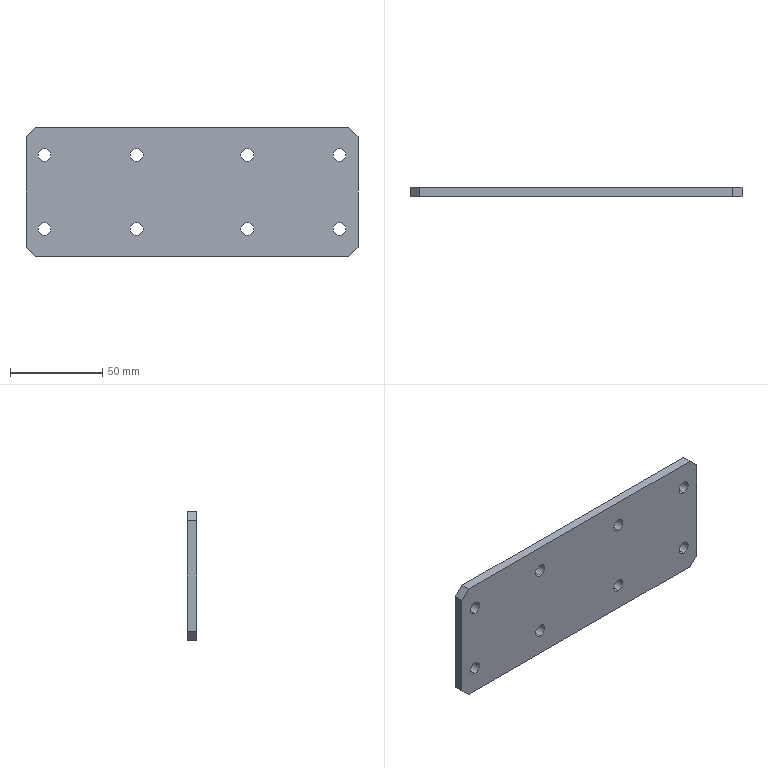Part | NX | features BREP 1 | 1 solid | 26 faces | box 180 x 5 x 70 mm | volume 61211 mm3 | cylinder 16 | plane 10 | commonest cylinder face diameters 7 x16
STEP:
#1=CARTESIAN_POINT('',(85.,5.,35.));
#2=VERTEX_POINT('',#1);
#3=CARTESIAN_POINT('',(90.,5.,30.));
#4=VERTEX_POINT('',#3);
#5=CARTESIAN_POINT('',(60.,5.,60.));
#6=DIRECTION('',(0.7071,0.,-0.7071));
#7=VECTOR('',#6,1000.);
#8=LINE('',#5,#7);
#9=EDGE_CURVE('',#2,#4,#8,.T.);
#10=ORIENTED_EDGE('',*,*,#9,.F.);
#11=CARTESIAN_POINT('',(85.,0.,35.));
#12=VERTEX_POINT('',#11);
#13=CARTESIAN_POINT('',(85.,5.,35.));
#14=DIRECTION('',(0.,1.,0.));
#15=VECTOR('',#14,1000.);
#16=LINE('',#13,#15);
#17=EDGE_CURVE('',#12,#2,#16,.T.);
#18=ORIENTED_EDGE('',*,*,#17,.F.);
#19=CARTESIAN_POINT('',(90.,0.,30.));
#20=VERTEX_POINT('',#19);
#21=CARTESIAN_POINT('',(90.,0.,30.));
#22=DIRECTION('',(-0.7071,0.,0.7071));
#23=VECTOR('',#22,1000.);
#24=LINE('',#21,#23);
#25=EDGE_CURVE('',#20,#12,#24,.T.);
#26=ORIENTED_EDGE('',*,*,#25,.F.);
#27=CARTESIAN_POINT('',(90.,5.,30.));
#28=DIRECTION('',(0.,-1.,0.));
#29=VECTOR('',#28,1000.);
#30=LINE('',#27,#29);
#31=EDGE_CURVE('',#4,#20,#30,.T.);
#32=ORIENTED_EDGE('',*,*,#31,.F.);
#33=EDGE_LOOP('',(#10,#18,#26,#32));
#34=FACE_BOUND('',#33,.T.);
#35=CARTESIAN_POINT('',(90.,5.,30.));
#36=DIRECTION('',(-0.7071,0.,-0.7071));
#37=DIRECTION('',(0.,-1.,0.));
#38=AXIS2_PLACEMENT_3D('',#35,#36,#37);
#39=PLANE('',#38);
#40=ADVANCED_FACE('',(#34),#39,.F.);
#41=CARTESIAN_POINT('',(90.,5.,-30.));
#42=VERTEX_POINT('',#41);
#43=CARTESIAN_POINT('',(85.,5.,-35.));
#44=VERTEX_POINT('',#43);
#45=CARTESIAN_POINT('',(60.,5.,-60.));
#46=DIRECTION('',(-0.7071,0.,-0.7071));
#47=VECTOR('',#46,1000.);
#48=LINE('',#45,#47);
#49=EDGE_CURVE('',#42,#44,#48,.T.);
#50=ORIENTED_EDGE('',*,*,#49,.F.);
#51=CARTESIAN_POINT('',(90.,0.,-30.));
#52=VERTEX_POINT('',#51);
#53=CARTESIAN_POINT('',(90.,5.,-30.));
#54=DIRECTION('',(0.,1.,0.));
#55=VECTOR('',#54,1000.);
#56=LINE('',#53,#55);
#57=EDGE_CURVE('',#52,#42,#56,.T.);
#58=ORIENTED_EDGE('',*,*,#57,.F.);
#59=CARTESIAN_POINT('',(85.,0.,-35.));
#60=VERTEX_POINT('',#59);
#61=CARTESIAN_POINT('',(85.,0.,-35.));
#62=DIRECTION('',(0.7071,0.,0.7071));
#63=VECTOR('',#62,1000.);
#64=LINE('',#61,#63);
#65=EDGE_CURVE('',#60,#52,#64,.T.);
#66=ORIENTED_EDGE('',*,*,#65,.F.);
#67=CARTESIAN_POINT('',(85.,5.,-35.));
#68=DIRECTION('',(0.,-1.,0.));
#69=VECTOR('',#68,1000.);
#70=LINE('',#67,#69);
#71=EDGE_CURVE('',#44,#60,#70,.T.);
#72=ORIENTED_EDGE('',*,*,#71,.F.);
#73=EDGE_LOOP('',(#50,#58,#66,#72));
#74=FACE_BOUND('',#73,.T.);
#75=CARTESIAN_POINT('',(85.,5.,-35.));
#76=DIRECTION('',(-0.7071,0.,0.7071));
#77=DIRECTION('',(0.,-1.,0.));
#78=AXIS2_PLACEMENT_3D('',#75,#76,#77);
#79=PLANE('',#78);
#80=ADVANCED_FACE('',(#74),#79,.F.);
#81=CARTESIAN_POINT('',(-90.,5.,30.));
#82=VERTEX_POINT('',#81);
#83=CARTESIAN_POINT('',(-85.,5.,35.));
#84=VERTEX_POINT('',#83);
#85=CARTESIAN_POINT('',(-60.,5.,60.));
#86=DIRECTION('',(0.7071,0.,0.7071));
#87=VECTOR('',#86,1000.);
#88=LINE('',#85,#87);
#89=EDGE_CURVE('',#82,#84,#88,.T.);
#90=ORIENTED_EDGE('',*,*,#89,.F.);
#91=CARTESIAN_POINT('',(-90.,0.,30.));
#92=VERTEX_POINT('',#91);
#93=CARTESIAN_POINT('',(-90.,5.,30.));
#94=DIRECTION('',(0.,1.,0.));
#95=VECTOR('',#94,1000.);
#96=LINE('',#93,#95);
#97=EDGE_CURVE('',#92,#82,#96,.T.);
#98=ORIENTED_EDGE('',*,*,#97,.F.);
#99=CARTESIAN_POINT('',(-85.,0.,35.));
#100=VERTEX_POINT('',#99);
#101=CARTESIAN_POINT('',(-85.,0.,35.));
#102=DIRECTION('',(-0.7071,0.,-0.7071));
#103=VECTOR('',#102,1000.);
#104=LINE('',#101,#103);
#105=EDGE_CURVE('',#100,#92,#104,.T.);
#106=ORIENTED_EDGE('',*,*,#105,.F.);
#107=CARTESIAN_POINT('',(-85.,5.,35.));
#108=DIRECTION('',(0.,-1.,0.));
#109=VECTOR('',#108,1000.);
#110=LINE('',#107,#109);
#111=EDGE_CURVE('',#84,#100,#110,.T.);
#112=ORIENTED_EDGE('',*,*,#111,.F.);
#113=EDGE_LOOP('',(#90,#98,#106,#112));
#114=FACE_BOUND('',#113,.T.);
#115=CARTESIAN_POINT('',(-85.,5.,35.));
#116=DIRECTION('',(0.7071,0.,-0.7071));
#117=DIRECTION('',(0.,-1.,0.));
#118=AXIS2_PLACEMENT_3D('',#115,#116,#117);
#119=PLANE('',#118);
#120=ADVANCED_FACE('',(#114),#119,.F.);
#121=CARTESIAN_POINT('',(-85.,5.,-35.));
#122=VERTEX_POINT('',#121);
#123=CARTESIAN_POINT('',(-90.,5.,-30.));
#124=VERTEX_POINT('',#123);
#125=CARTESIAN_POINT('',(-60.,5.,-60.));
#126=DIRECTION('',(-0.7071,0.,0.7071));
#127=VECTOR('',#126,1000.);
#128=LINE('',#125,#127);
#129=EDGE_CURVE('',#122,#124,#128,.T.);
#130=ORIENTED_EDGE('',*,*,#129,.F.);
#131=CARTESIAN_POINT('',(-85.,0.,-35.));
#132=VERTEX_POINT('',#131);
#133=CARTESIAN_POINT('',(-85.,5.,-35.));
#134=DIRECTION('',(0.,1.,0.));
#135=VECTOR('',#134,1000.);
#136=LINE('',#133,#135);
#137=EDGE_CURVE('',#132,#122,#136,.T.);
#138=ORIENTED_EDGE('',*,*,#137,.F.);
#139=CARTESIAN_POINT('',(-90.,0.,-30.));
#140=VERTEX_POINT('',#139);
#141=CARTESIAN_POINT('',(-90.,0.,-30.));
#142=DIRECTION('',(0.7071,0.,-0.7071));
#143=VECTOR('',#142,1000.);
#144=LINE('',#141,#143);
#145=EDGE_CURVE('',#140,#132,#144,.T.);
#146=ORIENTED_EDGE('',*,*,#145,.F.);
#147=CARTESIAN_POINT('',(-90.,5.,-30.));
#148=DIRECTION('',(0.,-1.,0.));
#149=VECTOR('',#148,1000.);
#150=LINE('',#147,#149);
#151=EDGE_CURVE('',#124,#140,#150,.T.);
#152=ORIENTED_EDGE('',*,*,#151,.F.);
#153=EDGE_LOOP('',(#130,#138,#146,#152));
#154=FACE_BOUND('',#153,.T.);
#155=CARTESIAN_POINT('',(-90.,5.,-30.));
#156=DIRECTION('',(0.7071,0.,0.7071));
#157=DIRECTION('',(0.,-1.,0.));
#158=AXIS2_PLACEMENT_3D('',#155,#156,#157);
#159=PLANE('',#158);
#160=ADVANCED_FACE('',(#154),#159,.F.);
#161=CARTESIAN_POINT('',(-80.,5.,-23.5));
#162=VERTEX_POINT('',#161);
#163=CARTESIAN_POINT('',(-80.,0.,-23.5));
#164=VERTEX_POINT('',#163);
#165=CARTESIAN_POINT('',(-80.,5.,-23.5));
#166=DIRECTION('',(0.,1.,0.));
#167=VECTOR('',#166,1000.);
#168=LINE('',#165,#167);
#169=EDGE_CURVE('',#162,#164,#168,.F.);
#170=ORIENTED_EDGE('',*,*,#169,.T.);
#171=CARTESIAN_POINT('',(-80.,0.,-16.5));
#172=VERTEX_POINT('',#171);
#173=CARTESIAN_POINT('',(-80.,0.,-20.));
#174=DIRECTION('',(0.,1.,0.));
#175=DIRECTION('',(0.,0.,1.));
#176=AXIS2_PLACEMENT_3D('',#173,#174,#175);
#177=CIRCLE('',#176,3.5);
#178=EDGE_CURVE('',#172,#164,#177,.T.);
#179=ORIENTED_EDGE('',*,*,#178,.F.);
#180=CARTESIAN_POINT('',(-80.,5.,-16.5));
#181=VERTEX_POINT('',#180);
#182=CARTESIAN_POINT('',(-80.,5.,-16.5));
#183=DIRECTION('',(0.,1.,0.));
#184=VECTOR('',#183,1000.);
#185=LINE('',#182,#184);
#186=EDGE_CURVE('',#181,#172,#185,.F.);
#187=ORIENTED_EDGE('',*,*,#186,.F.);
#188=CARTESIAN_POINT('',(-80.,5.,-20.));
#189=DIRECTION('',(0.,1.,0.));
#190=DIRECTION('',(0.,0.,1.));
#191=AXIS2_PLACEMENT_3D('',#188,#189,#190);
#192=CIRCLE('',#191,3.5);
#193=EDGE_CURVE('',#181,#162,#192,.T.);
#194=ORIENTED_EDGE('',*,*,#193,.T.);
#195=EDGE_LOOP('',(#170,#179,#187,#194));
#196=FACE_BOUND('',#195,.T.);
#197=CARTESIAN_POINT('',(-80.,5.,-20.));
#198=DIRECTION('',(0.,1.,0.));
#199=DIRECTION('',(0.,0.,1.));
#200=AXIS2_PLACEMENT_3D('',#197,#198,#199);
#201=CYLINDRICAL_SURFACE('',#200,3.5);
#202=ADVANCED_FACE('',(#196),#201,.F.);
#203=CARTESIAN_POINT('',(-30.,5.,-23.5));
#204=VERTEX_POINT('',#203);
#205=CARTESIAN_POINT('',(-30.,0.,-23.5));
#206=VERTEX_POINT('',#205);
#207=CARTESIAN_POINT('',(-30.,5.,-23.5));
#208=DIRECTION('',(0.,1.,0.));
#209=VECTOR('',#208,1000.);
#210=LINE('',#207,#209);
#211=EDGE_CURVE('',#204,#206,#210,.F.);
#212=ORIENTED_EDGE('',*,*,#211,.T.);
#213=CARTESIAN_POINT('',(-30.,0.,-16.5));
#214=VERTEX_POINT('',#213);
#215=CARTESIAN_POINT('',(-30.,0.,-20.));
#216=DIRECTION('',(0.,1.,0.));
#217=DIRECTION('',(0.,0.,1.));
#218=AXIS2_PLACEMENT_3D('',#215,#216,#217);
#219=CIRCLE('',#218,3.5);
#220=EDGE_CURVE('',#214,#206,#219,.T.);
#221=ORIENTED_EDGE('',*,*,#220,.F.);
#222=CARTESIAN_POINT('',(-30.,5.,-16.5));
#223=VERTEX_POINT('',#222);
#224=CARTESIAN_POINT('',(-30.,5.,-16.5));
#225=DIRECTION('',(0.,1.,0.));
#226=VECTOR('',#225,1000.);
#227=LINE('',#224,#226);
#228=EDGE_CURVE('',#223,#214,#227,.F.);
#229=ORIENTED_EDGE('',*,*,#228,.F.);
#230=CARTESIAN_POINT('',(-30.,5.,-20.));
#231=DIRECTION('',(0.,1.,0.));
#232=DIRECTION('',(0.,0.,1.));
#233=AXIS2_PLACEMENT_3D('',#230,#231,#232);
#234=CIRCLE('',#233,3.5);
#235=EDGE_CURVE('',#223,#204,#234,.T.);
#236=ORIENTED_EDGE('',*,*,#235,.T.);
#237=EDGE_LOOP('',(#212,#221,#229,#236));
#238=FACE_BOUND('',#237,.T.);
#239=CARTESIAN_POINT('',(-30.,5.,-20.));
#240=DIRECTION('',(0.,1.,0.));
#241=DIRECTION('',(0.,0.,1.));
#242=AXIS2_PLACEMENT_3D('',#239,#240,#241);
#243=CYLINDRICAL_SURFACE('',#242,3.5);
#244=ADVANCED_FACE('',(#238),#243,.F.);
#245=CARTESIAN_POINT('',(-80.,5.,16.5));
#246=VERTEX_POINT('',#245);
#247=CARTESIAN_POINT('',(-80.,0.,16.5));
#248=VERTEX_POINT('',#247);
#249=CARTESIAN_POINT('',(-80.,5.,16.5));
#250=DIRECTION('',(0.,1.,0.));
#251=VECTOR('',#250,1000.);
#252=LINE('',#249,#251);
#253=EDGE_CURVE('',#246,#248,#252,.F.);
#254=ORIENTED_EDGE('',*,*,#253,.T.);
#255=CARTESIAN_POINT('',(-80.,0.,23.5));
#256=VERTEX_POINT('',#255);
#257=CARTESIAN_POINT('',(-80.,0.,20.));
#258=DIRECTION('',(0.,1.,0.));
#259=DIRECTION('',(0.,0.,1.));
#260=AXIS2_PLACEMENT_3D('',#257,#258,#259);
#261=CIRCLE('',#260,3.5);
#262=EDGE_CURVE('',#256,#248,#261,.T.);
#263=ORIENTED_EDGE('',*,*,#262,.F.);
#264=CARTESIAN_POINT('',(-80.,5.,23.5));
#265=VERTEX_POINT('',#264);
#266=CARTESIAN_POINT('',(-80.,5.,23.5));
#267=DIRECTION('',(0.,1.,0.));
#268=VECTOR('',#267,1000.);
#269=LINE('',#266,#268);
#270=EDGE_CURVE('',#265,#256,#269,.F.);
#271=ORIENTED_EDGE('',*,*,#270,.F.);
#272=CARTESIAN_POINT('',(-80.,5.,20.));
#273=DIRECTION('',(0.,1.,0.));
#274=DIRECTION('',(0.,0.,1.));
#275=AXIS2_PLACEMENT_3D('',#272,#273,#274);
#276=CIRCLE('',#275,3.5);
#277=EDGE_CURVE('',#265,#246,#276,.T.);
#278=ORIENTED_EDGE('',*,*,#277,.T.);
#279=EDGE_LOOP('',(#254,#263,#271,#278));
#280=FACE_BOUND('',#279,.T.);
#281=CARTESIAN_POINT('',(-80.,5.,20.));
#282=DIRECTION('',(0.,1.,0.));
#283=DIRECTION('',(0.,0.,1.));
#284=AXIS2_PLACEMENT_3D('',#281,#282,#283);
#285=CYLINDRICAL_SURFACE('',#284,3.5);
#286=ADVANCED_FACE('',(#280),#285,.F.);
#287=CARTESIAN_POINT('',(-30.,5.,16.5));
#288=VERTEX_POINT('',#287);
#289=CARTESIAN_POINT('',(-30.,0.,16.5));
#290=VERTEX_POINT('',#289);
#291=CARTESIAN_POINT('',(-30.,5.,16.5));
#292=DIRECTION('',(0.,1.,0.));
#293=VECTOR('',#292,1000.);
#294=LINE('',#291,#293);
#295=EDGE_CURVE('',#288,#290,#294,.F.);
#296=ORIENTED_EDGE('',*,*,#295,.T.);
#297=CARTESIAN_POINT('',(-30.,0.,23.5));
#298=VERTEX_POINT('',#297);
#299=CARTESIAN_POINT('',(-30.,0.,20.));
#300=DIRECTION('',(0.,1.,0.));
#301=DIRECTION('',(0.,0.,1.));
#302=AXIS2_PLACEMENT_3D('',#299,#300,#301);
#303=CIRCLE('',#302,3.5);
#304=EDGE_CURVE('',#298,#290,#303,.T.);
#305=ORIENTED_EDGE('',*,*,#304,.F.);
#306=CARTESIAN_POINT('',(-30.,5.,23.5));
#307=VERTEX_POINT('',#306);
#308=CARTESIAN_POINT('',(-30.,5.,23.5));
#309=DIRECTION('',(0.,1.,0.));
#310=VECTOR('',#309,1000.);
#311=LINE('',#308,#310);
#312=EDGE_CURVE('',#307,#298,#311,.F.);
#313=ORIENTED_EDGE('',*,*,#312,.F.);
#314=CARTESIAN_POINT('',(-30.,5.,20.));
#315=DIRECTION('',(0.,1.,0.));
#316=DIRECTION('',(0.,0.,1.));
#317=AXIS2_PLACEMENT_3D('',#314,#315,#316);
#318=CIRCLE('',#317,3.5);
#319=EDGE_CURVE('',#307,#288,#318,.T.);
#320=ORIENTED_EDGE('',*,*,#319,.T.);
#321=EDGE_LOOP('',(#296,#305,#313,#320));
#322=FACE_BOUND('',#321,.T.);
#323=CARTESIAN_POINT('',(-30.,5.,20.));
#324=DIRECTION('',(0.,1.,0.));
#325=DIRECTION('',(0.,0.,1.));
#326=AXIS2_PLACEMENT_3D('',#323,#324,#325);
#327=CYLINDRICAL_SURFACE('',#326,3.5);
#328=ADVANCED_FACE('',(#322),#327,.F.);
#329=CARTESIAN_POINT('',(30.,5.,-23.5));
#330=VERTEX_POINT('',#329);
#331=CARTESIAN_POINT('',(30.,0.,-23.5));
#332=VERTEX_POINT('',#331);
#333=CARTESIAN_POINT('',(30.,5.,-23.5));
#334=DIRECTION('',(0.,1.,0.));
#335=VECTOR('',#334,1000.);
#336=LINE('',#333,#335);
#337=EDGE_CURVE('',#330,#332,#336,.F.);
#338=ORIENTED_EDGE('',*,*,#337,.T.);
#339=CARTESIAN_POINT('',(30.,0.,-16.5));
#340=VERTEX_POINT('',#339);
#341=CARTESIAN_POINT('',(30.,0.,-20.));
#342=DIRECTION('',(0.,1.,0.));
#343=DIRECTION('',(0.,0.,1.));
#344=AXIS2_PLACEMENT_3D('',#341,#342,#343);
#345=CIRCLE('',#344,3.5);
#346=EDGE_CURVE('',#340,#332,#345,.T.);
#347=ORIENTED_EDGE('',*,*,#346,.F.);
#348=CARTESIAN_POINT('',(30.,5.,-16.5));
#349=VERTEX_POINT('',#348);
#350=CARTESIAN_POINT('',(30.,5.,-16.5));
#351=DIRECTION('',(0.,1.,0.));
#352=VECTOR('',#351,1000.);
#353=LINE('',#350,#352);
#354=EDGE_CURVE('',#349,#340,#353,.F.);
#355=ORIENTED_EDGE('',*,*,#354,.F.);
#356=CARTESIAN_POINT('',(30.,5.,-20.));
#357=DIRECTION('',(0.,1.,0.));
#358=DIRECTION('',(0.,0.,1.));
#359=AXIS2_PLACEMENT_3D('',#356,#357,#358);
#360=CIRCLE('',#359,3.5);
#361=EDGE_CURVE('',#349,#330,#360,.T.);
#362=ORIENTED_EDGE('',*,*,#361,.T.);
#363=EDGE_LOOP('',(#338,#347,#355,#362));
#364=FACE_BOUND('',#363,.T.);
#365=CARTESIAN_POINT('',(30.,5.,-20.));
#366=DIRECTION('',(0.,1.,0.));
#367=DIRECTION('',(0.,0.,1.));
#368=AXIS2_PLACEMENT_3D('',#365,#366,#367);
#369=CYLINDRICAL_SURFACE('',#368,3.5);
#370=ADVANCED_FACE('',(#364),#369,.F.);
#371=CARTESIAN_POINT('',(30.,5.,16.5));
#372=VERTEX_POINT('',#371);
#373=CARTESIAN_POINT('',(30.,0.,16.5));
#374=VERTEX_POINT('',#373);
#375=CARTESIAN_POINT('',(30.,5.,16.5));
#376=DIRECTION('',(0.,1.,0.));
#377=VECTOR('',#376,1000.);
#378=LINE('',#375,#377);
#379=EDGE_CURVE('',#372,#374,#378,.F.);
#380=ORIENTED_EDGE('',*,*,#379,.T.);
#381=CARTESIAN_POINT('',(30.,0.,23.5));
#382=VERTEX_POINT('',#381);
#383=CARTESIAN_POINT('',(30.,0.,20.));
#384=DIRECTION('',(0.,1.,0.));
#385=DIRECTION('',(0.,0.,1.));
#386=AXIS2_PLACEMENT_3D('',#383,#384,#385);
#387=CIRCLE('',#386,3.5);
#388=EDGE_CURVE('',#382,#374,#387,.T.);
#389=ORIENTED_EDGE('',*,*,#388,.F.);
#390=CARTESIAN_POINT('',(30.,5.,23.5));
#391=VERTEX_POINT('',#390);
#392=CARTESIAN_POINT('',(30.,5.,23.5));
#393=DIRECTION('',(0.,1.,0.));
#394=VECTOR('',#393,1000.);
#395=LINE('',#392,#394);
#396=EDGE_CURVE('',#391,#382,#395,.F.);
#397=ORIENTED_EDGE('',*,*,#396,.F.);
#398=CARTESIAN_POINT('',(30.,5.,20.));
#399=DIRECTION('',(0.,1.,0.));
#400=DIRECTION('',(0.,0.,1.));
#401=AXIS2_PLACEMENT_3D('',#398,#399,#400);
#402=CIRCLE('',#401,3.5);
#403=EDGE_CURVE('',#391,#372,#402,.T.);
#404=ORIENTED_EDGE('',*,*,#403,.T.);
#405=EDGE_LOOP('',(#380,#389,#397,#404));
#406=FACE_BOUND('',#405,.T.);
#407=CARTESIAN_POINT('',(30.,5.,20.));
#408=DIRECTION('',(0.,1.,0.));
#409=DIRECTION('',(0.,0.,1.));
#410=AXIS2_PLACEMENT_3D('',#407,#408,#409);
#411=CYLINDRICAL_SURFACE('',#410,3.5);
#412=ADVANCED_FACE('',(#406),#411,.F.);
#413=CARTESIAN_POINT('',(80.,5.,-23.5));
#414=VERTEX_POINT('',#413);
#415=CARTESIAN_POINT('',(80.,0.,-23.5));
#416=VERTEX_POINT('',#415);
#417=CARTESIAN_POINT('',(80.,5.,-23.5));
#418=DIRECTION('',(0.,1.,0.));
#419=VECTOR('',#418,1000.);
#420=LINE('',#417,#419);
#421=EDGE_CURVE('',#414,#416,#420,.F.);
#422=ORIENTED_EDGE('',*,*,#421,.T.);
#423=CARTESIAN_POINT('',(80.,0.,-16.5));
#424=VERTEX_POINT('',#423);
#425=CARTESIAN_POINT('',(80.,0.,-20.));
#426=DIRECTION('',(0.,1.,0.));
#427=DIRECTION('',(0.,0.,1.));
#428=AXIS2_PLACEMENT_3D('',#425,#426,#427);
#429=CIRCLE('',#428,3.5);
#430=EDGE_CURVE('',#424,#416,#429,.T.);
#431=ORIENTED_EDGE('',*,*,#430,.F.);
#432=CARTESIAN_POINT('',(80.,5.,-16.5));
#433=VERTEX_POINT('',#432);
#434=CARTESIAN_POINT('',(80.,5.,-16.5));
#435=DIRECTION('',(0.,1.,0.));
#436=VECTOR('',#435,1000.);
#437=LINE('',#434,#436);
#438=EDGE_CURVE('',#433,#424,#437,.F.);
#439=ORIENTED_EDGE('',*,*,#438,.F.);
#440=CARTESIAN_POINT('',(80.,5.,-20.));
#441=DIRECTION('',(0.,1.,0.));
#442=DIRECTION('',(0.,0.,1.));
#443=AXIS2_PLACEMENT_3D('',#440,#441,#442);
#444=CIRCLE('',#443,3.5);
#445=EDGE_CURVE('',#433,#414,#444,.T.);
#446=ORIENTED_EDGE('',*,*,#445,.T.);
#447=EDGE_LOOP('',(#422,#431,#439,#446));
#448=FACE_BOUND('',#447,.T.);
#449=CARTESIAN_POINT('',(80.,5.,-20.));
#450=DIRECTION('',(0.,1.,0.));
#451=DIRECTION('',(0.,0.,1.));
#452=AXIS2_PLACEMENT_3D('',#449,#450,#451);
#453=CYLINDRICAL_SURFACE('',#452,3.5);
#454=ADVANCED_FACE('',(#448),#453,.F.);
#455=CARTESIAN_POINT('',(80.,5.,16.5));
#456=VERTEX_POINT('',#455);
#457=CARTESIAN_POINT('',(80.,0.,16.5));
#458=VERTEX_POINT('',#457);
#459=CARTESIAN_POINT('',(80.,5.,16.5));
#460=DIRECTION('',(0.,1.,0.));
#461=VECTOR('',#460,1000.);
#462=LINE('',#459,#461);
#463=EDGE_CURVE('',#456,#458,#462,.F.);
#464=ORIENTED_EDGE('',*,*,#463,.T.);
#465=CARTESIAN_POINT('',(80.,0.,23.5));
#466=VERTEX_POINT('',#465);
#467=CARTESIAN_POINT('',(80.,0.,20.));
#468=DIRECTION('',(0.,1.,0.));
#469=DIRECTION('',(0.,0.,1.));
#470=AXIS2_PLACEMENT_3D('',#467,#468,#469);
#471=CIRCLE('',#470,3.5);
#472=EDGE_CURVE('',#466,#458,#471,.T.);
#473=ORIENTED_EDGE('',*,*,#472,.F.);
#474=CARTESIAN_POINT('',(80.,5.,23.5));
#475=VERTEX_POINT('',#474);
#476=CARTESIAN_POINT('',(80.,5.,23.5));
#477=DIRECTION('',(0.,1.,0.));
#478=VECTOR('',#477,1000.);
#479=LINE('',#476,#478);
#480=EDGE_CURVE('',#475,#466,#479,.F.);
#481=ORIENTED_EDGE('',*,*,#480,.F.);
#482=CARTESIAN_POINT('',(80.,5.,20.));
#483=DIRECTION('',(0.,1.,0.));
#484=DIRECTION('',(0.,0.,1.));
#485=AXIS2_PLACEMENT_3D('',#482,#483,#484);
#486=CIRCLE('',#485,3.5);
#487=EDGE_CURVE('',#475,#456,#486,.T.);
#488=ORIENTED_EDGE('',*,*,#487,.T.);
#489=EDGE_LOOP('',(#464,#473,#481,#488));
#490=FACE_BOUND('',#489,.T.);
#491=CARTESIAN_POINT('',(80.,5.,20.));
#492=DIRECTION('',(0.,1.,0.));
#493=DIRECTION('',(0.,0.,1.));
#494=AXIS2_PLACEMENT_3D('',#491,#492,#493);
#495=CYLINDRICAL_SURFACE('',#494,3.5);
#496=ADVANCED_FACE('',(#490),#495,.F.);
#497=CARTESIAN_POINT('',(-90.,0.,35.));
#498=DIRECTION('',(0.,0.,1.));
#499=VECTOR('',#498,1000.);
#500=LINE('',#497,#499);
#501=EDGE_CURVE('',#140,#92,#500,.T.);
#502=ORIENTED_EDGE('',*,*,#501,.F.);
#503=ORIENTED_EDGE('',*,*,#145,.T.);
#504=CARTESIAN_POINT('',(90.,0.,-35.));
#505=DIRECTION('',(-1.,0.,0.));
#506=VECTOR('',#505,1000.);
#507=LINE('',#504,#506);
#508=EDGE_CURVE('',#60,#132,#507,.T.);
#509=ORIENTED_EDGE('',*,*,#508,.F.);
#510=ORIENTED_EDGE('',*,*,#65,.T.);
#511=CARTESIAN_POINT('',(90.,0.,35.));
#512=DIRECTION('',(0.,0.,-1.));
#513=VECTOR('',#512,1000.);
#514=LINE('',#511,#513);
#515=EDGE_CURVE('',#20,#52,#514,.T.);
#516=ORIENTED_EDGE('',*,*,#515,.F.);
#517=ORIENTED_EDGE('',*,*,#25,.T.);
#518=CARTESIAN_POINT('',(90.,0.,35.));
#519=DIRECTION('',(1.,0.,0.));
#520=VECTOR('',#519,1000.);
#521=LINE('',#518,#520);
#522=EDGE_CURVE('',#100,#12,#521,.T.);
#523=ORIENTED_EDGE('',*,*,#522,.F.);
#524=ORIENTED_EDGE('',*,*,#105,.T.);
#525=EDGE_LOOP('',(#502,#503,#509,#510,#516,#517,#523,#524));
#526=FACE_BOUND('',#525,.T.);
#527=ORIENTED_EDGE('',*,*,#472,.T.);
#528=CARTESIAN_POINT('',(80.,0.,20.));
#529=DIRECTION('',(0.,1.,0.));
#530=DIRECTION('',(0.,0.,1.));
#531=AXIS2_PLACEMENT_3D('',#528,#529,#530);
#532=CIRCLE('',#531,3.5);
#533=EDGE_CURVE('',#458,#466,#532,.T.);
#534=ORIENTED_EDGE('',*,*,#533,.T.);
#535=EDGE_LOOP('',(#527,#534));
#536=FACE_BOUND('',#535,.T.);
#537=ORIENTED_EDGE('',*,*,#430,.T.);
#538=CARTESIAN_POINT('',(80.,0.,-20.));
#539=DIRECTION('',(0.,1.,0.));
#540=DIRECTION('',(0.,0.,1.));
#541=AXIS2_PLACEMENT_3D('',#538,#539,#540);
#542=CIRCLE('',#541,3.5);
#543=EDGE_CURVE('',#416,#424,#542,.T.);
#544=ORIENTED_EDGE('',*,*,#543,.T.);
#545=EDGE_LOOP('',(#537,#544));
#546=FACE_BOUND('',#545,.T.);
#547=ORIENTED_EDGE('',*,*,#388,.T.);
#548=CARTESIAN_POINT('',(30.,0.,20.));
#549=DIRECTION('',(0.,1.,0.));
#550=DIRECTION('',(0.,0.,1.));
#551=AXIS2_PLACEMENT_3D('',#548,#549,#550);
#552=CIRCLE('',#551,3.5);
#553=EDGE_CURVE('',#374,#382,#552,.T.);
#554=ORIENTED_EDGE('',*,*,#553,.T.);
#555=EDGE_LOOP('',(#547,#554));
#556=FACE_BOUND('',#555,.T.);
#557=ORIENTED_EDGE('',*,*,#346,.T.);
#558=CARTESIAN_POINT('',(30.,0.,-20.));
#559=DIRECTION('',(0.,1.,0.));
#560=DIRECTION('',(0.,0.,1.));
#561=AXIS2_PLACEMENT_3D('',#558,#559,#560);
#562=CIRCLE('',#561,3.5);
#563=EDGE_CURVE('',#332,#340,#562,.T.);
#564=ORIENTED_EDGE('',*,*,#563,.T.);
#565=EDGE_LOOP('',(#557,#564));
#566=FACE_BOUND('',#565,.T.);
#567=ORIENTED_EDGE('',*,*,#304,.T.);
#568=CARTESIAN_POINT('',(-30.,0.,20.));
#569=DIRECTION('',(0.,1.,0.));
#570=DIRECTION('',(0.,0.,1.));
#571=AXIS2_PLACEMENT_3D('',#568,#569,#570);
#572=CIRCLE('',#571,3.5);
#573=EDGE_CURVE('',#290,#298,#572,.T.);
#574=ORIENTED_EDGE('',*,*,#573,.T.);
#575=EDGE_LOOP('',(#567,#574));
#576=FACE_BOUND('',#575,.T.);
#577=ORIENTED_EDGE('',*,*,#262,.T.);
#578=CARTESIAN_POINT('',(-80.,0.,20.));
#579=DIRECTION('',(0.,1.,0.));
#580=DIRECTION('',(0.,0.,1.));
#581=AXIS2_PLACEMENT_3D('',#578,#579,#580);
#582=CIRCLE('',#581,3.5);
#583=EDGE_CURVE('',#248,#256,#582,.T.);
#584=ORIENTED_EDGE('',*,*,#583,.T.);
#585=EDGE_LOOP('',(#577,#584));
#586=FACE_BOUND('',#585,.T.);
#587=ORIENTED_EDGE('',*,*,#220,.T.);
#588=CARTESIAN_POINT('',(-30.,0.,-20.));
#589=DIRECTION('',(0.,1.,0.));
#590=DIRECTION('',(0.,0.,1.));
#591=AXIS2_PLACEMENT_3D('',#588,#589,#590);
#592=CIRCLE('',#591,3.5);
#593=EDGE_CURVE('',#206,#214,#592,.T.);
#594=ORIENTED_EDGE('',*,*,#593,.T.);
#595=EDGE_LOOP('',(#587,#594));
#596=FACE_BOUND('',#595,.T.);
#597=ORIENTED_EDGE('',*,*,#178,.T.);
#598=CARTESIAN_POINT('',(-80.,0.,-20.));
#599=DIRECTION('',(0.,1.,0.));
#600=DIRECTION('',(0.,0.,1.));
#601=AXIS2_PLACEMENT_3D('',#598,#599,#600);
#602=CIRCLE('',#601,3.5);
#603=EDGE_CURVE('',#164,#172,#602,.T.);
#604=ORIENTED_EDGE('',*,*,#603,.T.);
#605=EDGE_LOOP('',(#597,#604));
#606=FACE_BOUND('',#605,.T.);
#607=CARTESIAN_POINT('',(0.,0.,0.));
#608=DIRECTION('',(0.,1.,0.));
#609=DIRECTION('',(0.,0.,1.));
#610=AXIS2_PLACEMENT_3D('',#607,#608,#609);
#611=PLANE('',#610);
#612=ADVANCED_FACE('',(#526,#536,#546,#556,#566,#576,#586,#596,#606),#611,.F.);
#613=CARTESIAN_POINT('',(90.,5.,-35.));
#614=DIRECTION('',(-1.,0.,0.));
#615=VECTOR('',#614,1000.);
#616=LINE('',#613,#615);
#617=EDGE_CURVE('',#44,#122,#616,.T.);
#618=ORIENTED_EDGE('',*,*,#617,.T.);
#619=ORIENTED_EDGE('',*,*,#129,.T.);
#620=CARTESIAN_POINT('',(-90.,5.,35.));
#621=DIRECTION('',(0.,0.,1.));
#622=VECTOR('',#621,1000.);
#623=LINE('',#620,#622);
#624=EDGE_CURVE('',#124,#82,#623,.T.);
#625=ORIENTED_EDGE('',*,*,#624,.T.);
#626=ORIENTED_EDGE('',*,*,#89,.T.);
#627=CARTESIAN_POINT('',(90.,5.,35.));
#628=DIRECTION('',(1.,0.,0.));
#629=VECTOR('',#628,1000.);
#630=LINE('',#627,#629);
#631=EDGE_CURVE('',#84,#2,#630,.T.);
#632=ORIENTED_EDGE('',*,*,#631,.T.);
#633=ORIENTED_EDGE('',*,*,#9,.T.);
#634=CARTESIAN_POINT('',(90.,5.,35.));
#635=DIRECTION('',(0.,0.,-1.));
#636=VECTOR('',#635,1000.);
#637=LINE('',#634,#636);
#638=EDGE_CURVE('',#4,#42,#637,.T.);
#639=ORIENTED_EDGE('',*,*,#638,.T.);
#640=ORIENTED_EDGE('',*,*,#49,.T.);
#641=EDGE_LOOP('',(#618,#619,#625,#626,#632,#633,#639,#640));
#642=FACE_BOUND('',#641,.T.);
#643=ORIENTED_EDGE('',*,*,#487,.F.);
#644=CARTESIAN_POINT('',(80.,5.,20.));
#645=DIRECTION('',(0.,1.,0.));
#646=DIRECTION('',(0.,0.,1.));
#647=AXIS2_PLACEMENT_3D('',#644,#645,#646);
#648=CIRCLE('',#647,3.5);
#649=EDGE_CURVE('',#456,#475,#648,.T.);
#650=ORIENTED_EDGE('',*,*,#649,.F.);
#651=EDGE_LOOP('',(#643,#650));
#652=FACE_BOUND('',#651,.T.);
#653=ORIENTED_EDGE('',*,*,#445,.F.);
#654=CARTESIAN_POINT('',(80.,5.,-20.));
#655=DIRECTION('',(0.,1.,0.));
#656=DIRECTION('',(0.,0.,1.));
#657=AXIS2_PLACEMENT_3D('',#654,#655,#656);
#658=CIRCLE('',#657,3.5);
#659=EDGE_CURVE('',#414,#433,#658,.T.);
#660=ORIENTED_EDGE('',*,*,#659,.F.);
#661=EDGE_LOOP('',(#653,#660));
#662=FACE_BOUND('',#661,.T.);
#663=ORIENTED_EDGE('',*,*,#403,.F.);
#664=CARTESIAN_POINT('',(30.,5.,20.));
#665=DIRECTION('',(0.,1.,0.));
#666=DIRECTION('',(0.,0.,1.));
#667=AXIS2_PLACEMENT_3D('',#664,#665,#666);
#668=CIRCLE('',#667,3.5);
#669=EDGE_CURVE('',#372,#391,#668,.T.);
#670=ORIENTED_EDGE('',*,*,#669,.F.);
#671=EDGE_LOOP('',(#663,#670));
#672=FACE_BOUND('',#671,.T.);
#673=ORIENTED_EDGE('',*,*,#361,.F.);
#674=CARTESIAN_POINT('',(30.,5.,-20.));
#675=DIRECTION('',(0.,1.,0.));
#676=DIRECTION('',(0.,0.,1.));
#677=AXIS2_PLACEMENT_3D('',#674,#675,#676);
#678=CIRCLE('',#677,3.5);
#679=EDGE_CURVE('',#330,#349,#678,.T.);
#680=ORIENTED_EDGE('',*,*,#679,.F.);
#681=EDGE_LOOP('',(#673,#680));
#682=FACE_BOUND('',#681,.T.);
#683=ORIENTED_EDGE('',*,*,#319,.F.);
#684=CARTESIAN_POINT('',(-30.,5.,20.));
#685=DIRECTION('',(0.,1.,0.));
#686=DIRECTION('',(0.,0.,1.));
#687=AXIS2_PLACEMENT_3D('',#684,#685,#686);
#688=CIRCLE('',#687,3.5);
#689=EDGE_CURVE('',#288,#307,#688,.T.);
#690=ORIENTED_EDGE('',*,*,#689,.F.);
#691=EDGE_LOOP('',(#683,#690));
#692=FACE_BOUND('',#691,.T.);
#693=ORIENTED_EDGE('',*,*,#277,.F.);
#694=CARTESIAN_POINT('',(-80.,5.,20.));
#695=DIRECTION('',(0.,1.,0.));
#696=DIRECTION('',(0.,0.,1.));
#697=AXIS2_PLACEMENT_3D('',#694,#695,#696);
#698=CIRCLE('',#697,3.5);
#699=EDGE_CURVE('',#246,#265,#698,.T.);
#700=ORIENTED_EDGE('',*,*,#699,.F.);
#701=EDGE_LOOP('',(#693,#700));
#702=FACE_BOUND('',#701,.T.);
#703=ORIENTED_EDGE('',*,*,#235,.F.);
#704=CARTESIAN_POINT('',(-30.,5.,-20.));
#705=DIRECTION('',(0.,1.,0.));
#706=DIRECTION('',(0.,0.,1.));
#707=AXIS2_PLACEMENT_3D('',#704,#705,#706);
#708=CIRCLE('',#707,3.5);
#709=EDGE_CURVE('',#204,#223,#708,.T.);
#710=ORIENTED_EDGE('',*,*,#709,.F.);
#711=EDGE_LOOP('',(#703,#710));
#712=FACE_BOUND('',#711,.T.);
#713=ORIENTED_EDGE('',*,*,#193,.F.);
#714=CARTESIAN_POINT('',(-80.,5.,-20.));
#715=DIRECTION('',(0.,1.,0.));
#716=DIRECTION('',(0.,0.,1.));
#717=AXIS2_PLACEMENT_3D('',#714,#715,#716);
#718=CIRCLE('',#717,3.5);
#719=EDGE_CURVE('',#162,#181,#718,.T.);
#720=ORIENTED_EDGE('',*,*,#719,.F.);
#721=EDGE_LOOP('',(#713,#720));
#722=FACE_BOUND('',#721,.T.);
#723=CARTESIAN_POINT('',(0.,5.,0.));
#724=DIRECTION('',(0.,1.,0.));
#725=DIRECTION('',(0.,0.,1.));
#726=AXIS2_PLACEMENT_3D('',#723,#724,#725);
#727=PLANE('',#726);
#728=ADVANCED_FACE('',(#642,#652,#662,#672,#682,#692,#702,#712,#722),#727,.T.);
#729=ORIENTED_EDGE('',*,*,#508,.T.);
#730=ORIENTED_EDGE('',*,*,#137,.T.);
#731=ORIENTED_EDGE('',*,*,#617,.F.);
#732=ORIENTED_EDGE('',*,*,#71,.T.);
#733=EDGE_LOOP('',(#729,#730,#731,#732));
#734=FACE_BOUND('',#733,.T.);
#735=CARTESIAN_POINT('',(90.,5.,-35.));
#736=DIRECTION('',(0.,0.,1.));
#737=DIRECTION('',(1.,0.,0.));
#738=AXIS2_PLACEMENT_3D('',#735,#736,#737);
#739=PLANE('',#738);
#740=ADVANCED_FACE('',(#734),#739,.F.);
#741=ORIENTED_EDGE('',*,*,#515,.T.);
#742=ORIENTED_EDGE('',*,*,#57,.T.);
#743=ORIENTED_EDGE('',*,*,#638,.F.);
#744=ORIENTED_EDGE('',*,*,#31,.T.);
#745=EDGE_LOOP('',(#741,#742,#743,#744));
#746=FACE_BOUND('',#745,.T.);
#747=CARTESIAN_POINT('',(90.,5.,35.));
#748=DIRECTION('',(-1.,0.,0.));
#749=DIRECTION('',(0.,0.,1.));
#750=AXIS2_PLACEMENT_3D('',#747,#748,#749);
#751=PLANE('',#750);
#752=ADVANCED_FACE('',(#746),#751,.F.);
#753=ORIENTED_EDGE('',*,*,#631,.F.);
#754=ORIENTED_EDGE('',*,*,#111,.T.);
#755=ORIENTED_EDGE('',*,*,#522,.T.);
#756=ORIENTED_EDGE('',*,*,#17,.T.);
#757=EDGE_LOOP('',(#753,#754,#755,#756));
#758=FACE_BOUND('',#757,.T.);
#759=CARTESIAN_POINT('',(90.,5.,35.));
#760=DIRECTION('',(0.,0.,-1.));
#761=DIRECTION('',(-1.,0.,0.));
#762=AXIS2_PLACEMENT_3D('',#759,#760,#761);
#763=PLANE('',#762);
#764=ADVANCED_FACE('',(#758),#763,.F.);
#765=ORIENTED_EDGE('',*,*,#624,.F.);
#766=ORIENTED_EDGE('',*,*,#151,.T.);
#767=ORIENTED_EDGE('',*,*,#501,.T.);
#768=ORIENTED_EDGE('',*,*,#97,.T.);
#769=EDGE_LOOP('',(#765,#766,#767,#768));
#770=FACE_BOUND('',#769,.T.);
#771=CARTESIAN_POINT('',(-90.,5.,35.));
#772=DIRECTION('',(1.,0.,0.));
#773=DIRECTION('',(0.,0.,-1.));
#774=AXIS2_PLACEMENT_3D('',#771,#772,#773);
#775=PLANE('',#774);
#776=ADVANCED_FACE('',(#770),#775,.F.);
#777=ORIENTED_EDGE('',*,*,#533,.F.);
#778=ORIENTED_EDGE('',*,*,#463,.F.);
#779=ORIENTED_EDGE('',*,*,#649,.T.);
#780=ORIENTED_EDGE('',*,*,#480,.T.);
#781=EDGE_LOOP('',(#777,#778,#779,#780));
#782=FACE_BOUND('',#781,.T.);
#783=CARTESIAN_POINT('',(80.,5.,20.));
#784=DIRECTION('',(0.,1.,0.));
#785=DIRECTION('',(0.,0.,1.));
#786=AXIS2_PLACEMENT_3D('',#783,#784,#785);
#787=CYLINDRICAL_SURFACE('',#786,3.5);
#788=ADVANCED_FACE('',(#782),#787,.F.);
#789=ORIENTED_EDGE('',*,*,#543,.F.);
#790=ORIENTED_EDGE('',*,*,#421,.F.);
#791=ORIENTED_EDGE('',*,*,#659,.T.);
#792=ORIENTED_EDGE('',*,*,#438,.T.);
#793=EDGE_LOOP('',(#789,#790,#791,#792));
#794=FACE_BOUND('',#793,.T.);
#795=CARTESIAN_POINT('',(80.,5.,-20.));
#796=DIRECTION('',(0.,1.,0.));
#797=DIRECTION('',(0.,0.,1.));
#798=AXIS2_PLACEMENT_3D('',#795,#796,#797);
#799=CYLINDRICAL_SURFACE('',#798,3.5);
#800=ADVANCED_FACE('',(#794),#799,.F.);
#801=ORIENTED_EDGE('',*,*,#553,.F.);
#802=ORIENTED_EDGE('',*,*,#379,.F.);
#803=ORIENTED_EDGE('',*,*,#669,.T.);
#804=ORIENTED_EDGE('',*,*,#396,.T.);
#805=EDGE_LOOP('',(#801,#802,#803,#804));
#806=FACE_BOUND('',#805,.T.);
#807=CARTESIAN_POINT('',(30.,5.,20.));
#808=DIRECTION('',(0.,1.,0.));
#809=DIRECTION('',(0.,0.,1.));
#810=AXIS2_PLACEMENT_3D('',#807,#808,#809);
#811=CYLINDRICAL_SURFACE('',#810,3.5);
#812=ADVANCED_FACE('',(#806),#811,.F.);
#813=ORIENTED_EDGE('',*,*,#563,.F.);
#814=ORIENTED_EDGE('',*,*,#337,.F.);
#815=ORIENTED_EDGE('',*,*,#679,.T.);
#816=ORIENTED_EDGE('',*,*,#354,.T.);
#817=EDGE_LOOP('',(#813,#814,#815,#816));
#818=FACE_BOUND('',#817,.T.);
#819=CARTESIAN_POINT('',(30.,5.,-20.));
#820=DIRECTION('',(0.,1.,0.));
#821=DIRECTION('',(0.,0.,1.));
#822=AXIS2_PLACEMENT_3D('',#819,#820,#821);
#823=CYLINDRICAL_SURFACE('',#822,3.5);
#824=ADVANCED_FACE('',(#818),#823,.F.);
#825=ORIENTED_EDGE('',*,*,#573,.F.);
#826=ORIENTED_EDGE('',*,*,#295,.F.);
#827=ORIENTED_EDGE('',*,*,#689,.T.);
#828=ORIENTED_EDGE('',*,*,#312,.T.);
#829=EDGE_LOOP('',(#825,#826,#827,#828));
#830=FACE_BOUND('',#829,.T.);
#831=CARTESIAN_POINT('',(-30.,5.,20.));
#832=DIRECTION('',(0.,1.,0.));
#833=DIRECTION('',(0.,0.,1.));
#834=AXIS2_PLACEMENT_3D('',#831,#832,#833);
#835=CYLINDRICAL_SURFACE('',#834,3.5);
#836=ADVANCED_FACE('',(#830),#835,.F.);
#837=ORIENTED_EDGE('',*,*,#583,.F.);
#838=ORIENTED_EDGE('',*,*,#253,.F.);
#839=ORIENTED_EDGE('',*,*,#699,.T.);
#840=ORIENTED_EDGE('',*,*,#270,.T.);
#841=EDGE_LOOP('',(#837,#838,#839,#840));
#842=FACE_BOUND('',#841,.T.);
#843=CARTESIAN_POINT('',(-80.,5.,20.));
#844=DIRECTION('',(0.,1.,0.));
#845=DIRECTION('',(0.,0.,1.));
#846=AXIS2_PLACEMENT_3D('',#843,#844,#845);
#847=CYLINDRICAL_SURFACE('',#846,3.5);
#848=ADVANCED_FACE('',(#842),#847,.F.);
#849=ORIENTED_EDGE('',*,*,#593,.F.);
#850=ORIENTED_EDGE('',*,*,#211,.F.);
#851=ORIENTED_EDGE('',*,*,#709,.T.);
#852=ORIENTED_EDGE('',*,*,#228,.T.);
#853=EDGE_LOOP('',(#849,#850,#851,#852));
#854=FACE_BOUND('',#853,.T.);
#855=CARTESIAN_POINT('',(-30.,5.,-20.));
#856=DIRECTION('',(0.,1.,0.));
#857=DIRECTION('',(0.,0.,1.));
#858=AXIS2_PLACEMENT_3D('',#855,#856,#857);
#859=CYLINDRICAL_SURFACE('',#858,3.5);
#860=ADVANCED_FACE('',(#854),#859,.F.);
#861=ORIENTED_EDGE('',*,*,#603,.F.);
#862=ORIENTED_EDGE('',*,*,#169,.F.);
#863=ORIENTED_EDGE('',*,*,#719,.T.);
#864=ORIENTED_EDGE('',*,*,#186,.T.);
#865=EDGE_LOOP('',(#861,#862,#863,#864));
#866=FACE_BOUND('',#865,.T.);
#867=CARTESIAN_POINT('',(-80.,5.,-20.));
#868=DIRECTION('',(0.,1.,0.));
#869=DIRECTION('',(0.,0.,1.));
#870=AXIS2_PLACEMENT_3D('',#867,#868,#869);
#871=CYLINDRICAL_SURFACE('',#870,3.5);
#872=ADVANCED_FACE('',(#866),#871,.F.);
#873=CLOSED_SHELL('',(#40,#80,#120,#160,#202,#244,#286,#328,#370,#412,#454,#496,#612,#728,#740,#752,#764,#776,#788,#800,#812,#824,#836,#848,#860,#872));
#874=MANIFOLD_SOLID_BREP('',#873);
#875=(LENGTH_UNIT()NAMED_UNIT(*)SI_UNIT(.MILLI.,.METRE.));
#876=UNCERTAINTY_MEASURE_WITH_UNIT(LENGTH_MEASURE(0.00001),#875,'','');
#877=(NAMED_UNIT(*)PLANE_ANGLE_UNIT()SI_UNIT($,.RADIAN.));
#878=(NAMED_UNIT(*)SI_UNIT($,.STERADIAN.)SOLID_ANGLE_UNIT());
#879=(GEOMETRIC_REPRESENTATION_CONTEXT(3)GLOBAL_UNCERTAINTY_ASSIGNED_CONTEXT((#876))GLOBAL_UNIT_ASSIGNED_CONTEXT((#875,#877,#878))REPRESENTATION_CONTEXT('',''));
#880=ADVANCED_BREP_SHAPE_REPRESENTATION('',(#874),#879);